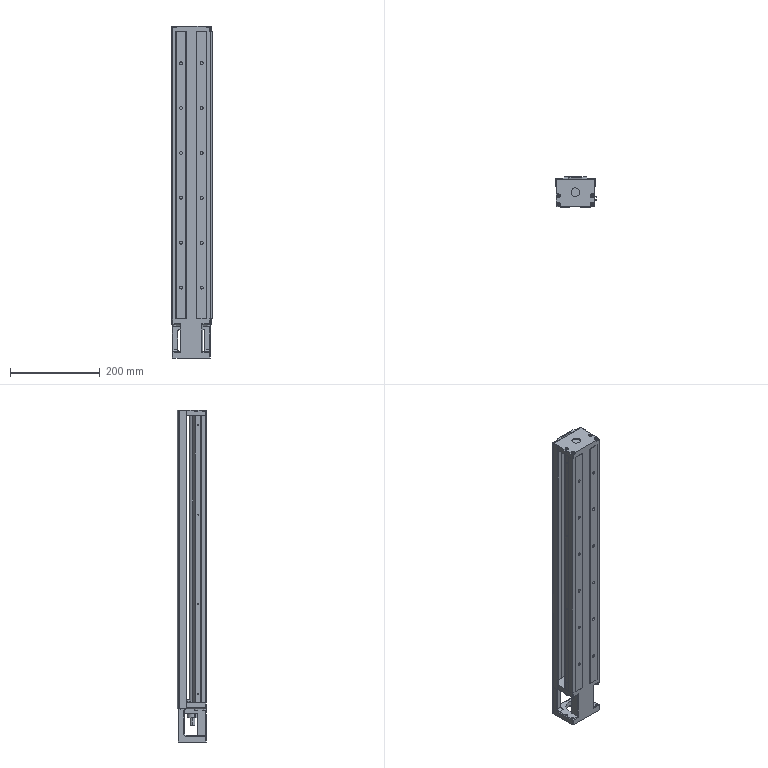Part | STEP file | Single-axis module KK86D20C-640A1 rail | 3 solids | 517 faces | box 91 x 66.1 x 740 mm | volume 1447493 mm3 | plane 262 | cylinder 215 | cone 26 | spline 14 | commonest cylinder face diameters 3 x37 4.5 x24 6.6 x24 7.5 x24 11 x24 2.15 x16